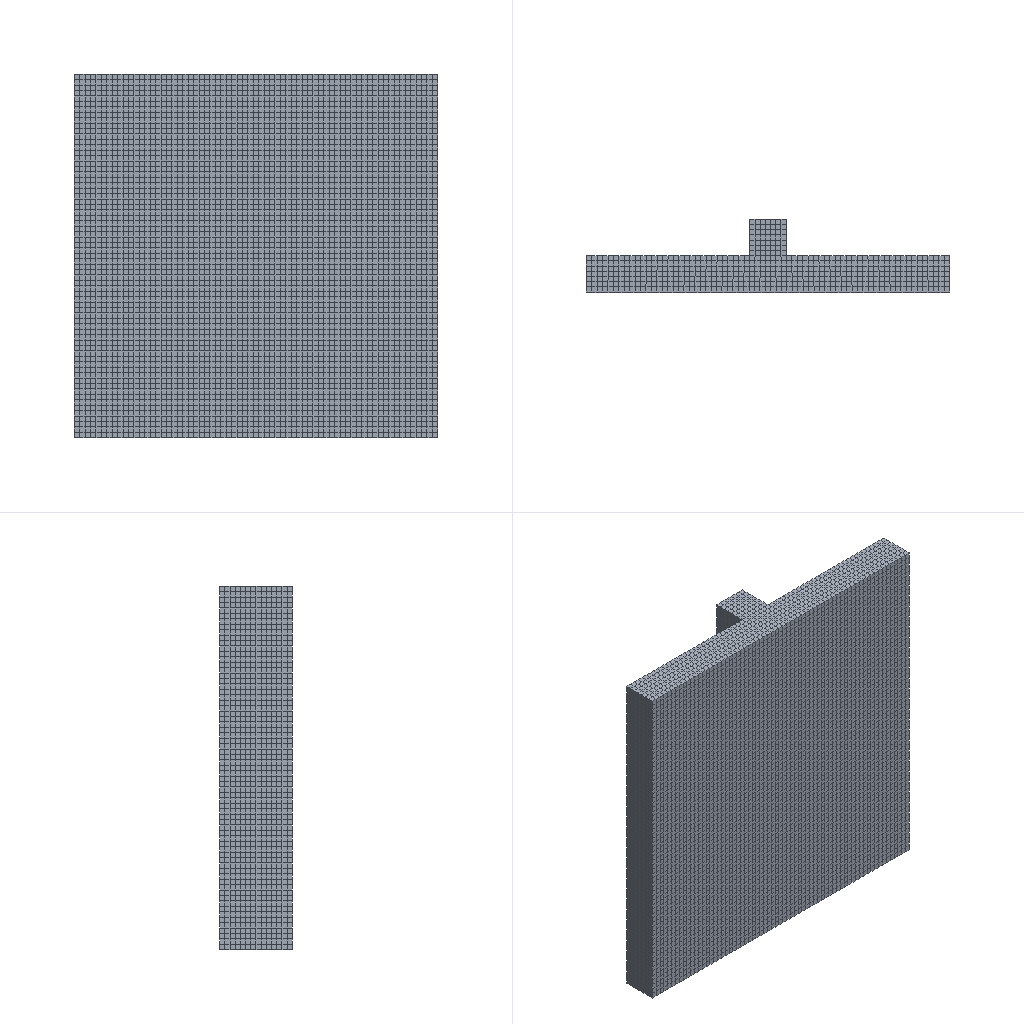Simulation study | abaqus
Set-up summary, first 153 of 190 lines:
category,name,step,type,value,unit,region
solver,abaqus,,Abaqus/CAE 2024
units,mm-N-s-tonne (MPa),,inferred,E= density=7.8e-09
analysis,Step-1,,heat transfer,time_period=2.76
analysis,Step-2,,heat transfer,time_period=50
mesh,nodes,,,40800
mesh,elements,,,34706
element_type,DC3D8,,,34706
material,Material-1,,density,7.8e-09
material,Material-1,,conductivity,17.5
material,Material-1,,specific_heat,5.13e+08
material,Material-1,,behaviors,conductivity; specific heat
section,Material-1,,solid section,,,Set-1
load,Predefined,initial,initial condition temperature
load,Load-1,Step-1,dflux,3.23768e-290,,Part-1-1.316
load,Load-1,Step-1,dflux,2.36258e-281,,Part-1-1.316
load,Load-1,Step-1,dflux,4.91222e-276,,Part-1-1.316
load,Load-1,Step-1,dflux,2.9101e-274,,Part-1-1.316
load,Load-1,Step-1,dflux,4.91222e-276,,Part-1-1.316
load,Load-1,Step-1,dflux,2.36258e-281,,Part-1-1.316
load,Load-1,Step-1,dflux,3.23768e-290,,Part-1-1.316
load,Load-1,Step-1,dflux,1.0318e-245,,Part-1-1.316
load,Load-1,Step-1,dflux,7.52918e-237,,Part-1-1.316
load,Load-1,Step-1,dflux,1.56545e-231,,Part-1-1.316
load,Load-1,Step-1,dflux,9.27406e-230,,Part-1-1.316
load,Load-1,Step-1,dflux,1.56545e-231,,Part-1-1.316
load,Load-1,Step-1,dflux,7.52918e-237,,Part-1-1.316
load,Load-1,Step-1,dflux,1.0318e-245,,Part-1-1.316
load,Load-1,Step-1,dflux,4.43605e-205,,Part-1-1.316
load,Load-1,Step-1,dflux,3.23705e-196,,Part-1-1.316
load,Load-1,Step-1,dflux,6.7304e-191,,Part-1-1.316
load,Load-1,Step-1,dflux,3.98723e-189,,Part-1-1.316
load,Load-1,Step-1,dflux,6.7304e-191,,Part-1-1.316
load,Load-1,Step-1,dflux,3.23705e-196,,Part-1-1.316
load,Load-1,Step-1,dflux,4.43605e-205,,Part-1-1.316
load,Load-1,Step-1,dflux,2.57396e-168,,Part-1-1.316
load,Load-1,Step-1,dflux,1.87825e-159,,Part-1-1.316
load,Load-1,Step-1,dflux,3.90522e-154,,Part-1-1.316
load,Load-1,Step-1,dflux,2.31353e-152,,Part-1-1.316
load,Load-1,Step-1,dflux,3.90522e-154,,Part-1-1.316
load,Load-1,Step-1,dflux,1.87825e-159,,Part-1-1.316
load,Load-1,Step-1,dflux,2.57396e-168,,Part-1-1.316
load,Load-1,Step-1,dflux,2.01555e-135,,Part-1-1.316
load,Load-1,Step-1,dflux,1.47078e-126,,Part-1-1.316
load,Load-1,Step-1,dflux,3.05801e-121,,Part-1-1.316
load,Load-1,Step-1,dflux,1.81163e-119,,Part-1-1.316
load,Load-1,Step-1,dflux,3.05801e-121,,Part-1-1.316
load,Load-1,Step-1,dflux,1.47078e-126,,Part-1-1.316
load,Load-1,Step-1,dflux,2.01555e-135,,Part-1-1.316
load,Load-1,Step-1,dflux,2.12957e-106,,Part-1-1.316
load,Load-1,Step-1,dflux,1.55398e-97,,Part-1-1.316
load,Load-1,Step-1,dflux,3.231e-92,,Part-1-1.316
load,Load-1,Step-1,dflux,1.91411e-90,,Part-1-1.316
load,Load-1,Step-1,dflux,3.231e-92,,Part-1-1.316
load,Load-1,Step-1,dflux,1.55398e-97,,Part-1-1.316
load,Load-1,Step-1,dflux,2.12957e-106,,Part-1-1.316
load,Load-1,Step-1,dflux,3.03647e-81,,Part-1-1.316
load,Load-1,Step-1,dflux,2.21575e-72,,Part-1-1.316
load,Load-1,Step-1,dflux,4.60694e-67,,Part-1-1.316
load,Load-1,Step-1,dflux,2.72925e-65,,Part-1-1.316
load,Load-1,Step-1,dflux,4.60694e-67,,Part-1-1.316
load,Load-1,Step-1,dflux,2.21575e-72,,Part-1-1.316
load,Load-1,Step-1,dflux,3.03647e-81,,Part-1-1.316
load,Load-1,Step-1,dflux,5.84197e-60,,Part-1-1.316
load,Load-1,Step-1,dflux,4.26297e-51,,Part-1-1.316
load,Load-1,Step-1,dflux,8.86347e-46,,Part-1-1.316
load,Load-1,Step-1,dflux,5.2509e-44,,Part-1-1.316
load,Load-1,Step-1,dflux,8.86347e-46,,Part-1-1.316
load,Load-1,Step-1,dflux,4.26297e-51,,Part-1-1.316
load,Load-1,Step-1,dflux,5.84197e-60,,Part-1-1.316
load,Load-1,Step-1,dflux,1.5167e-42,,Part-1-1.316
load,Load-1,Step-1,dflux,1.10676e-33,,Part-1-1.316
load,Load-1,Step-1,dflux,2.30114e-28,,Part-1-1.316
load,Load-1,Step-1,dflux,1.36324e-26,,Part-1-1.316
load,Load-1,Step-1,dflux,2.30114e-28,,Part-1-1.316
load,Load-1,Step-1,dflux,1.10676e-33,,Part-1-1.316
load,Load-1,Step-1,dflux,1.5167e-42,,Part-1-1.316
load,Load-1,Step-1,dflux,5.31377e-29,,Part-1-1.316
load,Load-1,Step-1,dflux,3.87753e-20,,Part-1-1.316
load,Load-1,Step-1,dflux,8.06207e-15,,Part-1-1.316
load,Load-1,Step-1,dflux,4.77614e-13,,Part-1-1.316
load,Load-1,Step-1,dflux,8.06207e-15,,Part-1-1.316
load,Load-1,Step-1,dflux,3.87753e-20,,Part-1-1.316
load,Load-1,Step-1,dflux,5.31377e-29,,Part-1-1.316
load,Load-1,Step-1,dflux,2.51209e-19,,Part-1-1.316
load,Load-1,Step-1,dflux,1.83311e-10,,Part-1-1.316
load,Load-1,Step-1,dflux,3.81135e-05,,Part-1-1.316
load,Load-1,Step-1,dflux,0.002258,,Part-1-1.316
load,Load-1,Step-1,dflux,3.81135e-05,,Part-1-1.316
load,Load-1,Step-1,dflux,1.83311e-10,,Part-1-1.316
load,Load-1,Step-1,dflux,2.51209e-19,,Part-1-1.316
load,Load-1,Step-1,dflux,1.60257e-13,,Part-1-1.316
load,Load-1,Step-1,dflux,0.0001169,,Part-1-1.316
load,Load-1,Step-1,dflux,24.314,,Part-1-1.317
load,Load-1,Step-1,dflux,1440.43,,Part-1-1.317
load,Load-1,Step-1,dflux,24.314,,Part-1-1.317
load,Load-1,Step-1,dflux,0.0001169,,Part-1-1.317
load,Load-1,Step-1,dflux,1.60257e-13,,Part-1-1.317
load,Load-1,Step-1,dflux,1.37958e-11,,Part-1-1.317
load,Load-1,Step-1,dflux,0.01007,,Part-1-1.317
load,Load-1,Step-1,dflux,2093.11,,Part-1-1.317
load,Load-1,Step-1,dflux,124000,,Part-1-1.317
load,Load-1,Step-1,dflux,2093.11,,Part-1-1.317
load,Load-1,Step-1,dflux,0.01007,,Part-1-1.317
load,Load-1,Step-1,dflux,1.37958e-11,,Part-1-1.317
load,Load-1,Step-1,dflux,1.60257e-13,,Part-1-1.317
load,Load-1,Step-1,dflux,0.0001169,,Part-1-1.317
load,Load-1,Step-1,dflux,24.314,,Part-1-1.317
load,Load-1,Step-1,dflux,1440.43,,Part-1-1.317
load,Load-1,Step-1,dflux,24.314,,Part-1-1.317
load,Load-1,Step-1,dflux,0.0001169,,Part-1-1.317
load,Load-1,Step-1,dflux,1.60257e-13,,Part-1-1.317
load,Load-1,Step-1,dflux,2.51209e-19,,Part-1-1.317
load,Load-1,Step-1,dflux,1.83311e-10,,Part-1-1.317
load,Load-1,Step-1,dflux,3.81135e-05,,Part-1-1.317
load,Load-1,Step-1,dflux,0.002258,,Part-1-1.317
load,Load-1,Step-1,dflux,3.81135e-05,,Part-1-1.317
load,Load-1,Step-1,dflux,1.83311e-10,,Part-1-1.317
load,Load-1,Step-1,dflux,2.51209e-19,,Part-1-1.317
load,Load-1,Step-1,dflux,5.31377e-29,,Part-1-1.317
load,Load-1,Step-1,dflux,3.87753e-20,,Part-1-1.317
load,Load-1,Step-1,dflux,8.06207e-15,,Part-1-1.317
load,Load-1,Step-1,dflux,4.77614e-13,,Part-1-1.317
load,Load-1,Step-1,dflux,8.06207e-15,,Part-1-1.317
load,Load-1,Step-1,dflux,3.87753e-20,,Part-1-1.317
load,Load-1,Step-1,dflux,5.31377e-29,,Part-1-1.317
load,Load-1,Step-1,dflux,1.5167e-42,,Part-1-1.317
load,Load-1,Step-1,dflux,1.10676e-33,,Part-1-1.317
load,Load-1,Step-1,dflux,2.30114e-28,,Part-1-1.317
load,Load-1,Step-1,dflux,1.36324e-26,,Part-1-1.317
load,Load-1,Step-1,dflux,2.30114e-28,,Part-1-1.317
load,Load-1,Step-1,dflux,1.10676e-33,,Part-1-1.317
load,Load-1,Step-1,dflux,1.5167e-42,,Part-1-1.317
load,Load-1,Step-1,dflux,5.84197e-60,,Part-1-1.317
load,Load-1,Step-1,dflux,4.26297e-51,,Part-1-1.317
load,Load-1,Step-1,dflux,8.86347e-46,,Part-1-1.317
load,Load-1,Step-1,dflux,5.2509e-44,,Part-1-1.317
load,Load-1,Step-1,dflux,8.86347e-46,,Part-1-1.317
load,Load-1,Step-1,dflux,4.26297e-51,,Part-1-1.317
load,Load-1,Step-1,dflux,5.84197e-60,,Part-1-1.317
load,Load-1,Step-1,dflux,3.03647e-81,,Part-1-1.317
load,Load-1,Step-1,dflux,2.21575e-72,,Part-1-1.317
load,Load-1,Step-1,dflux,4.60694e-67,,Part-1-1.317
load,Load-1,Step-1,dflux,2.72925e-65,,Part-1-1.317
load,Load-1,Step-1,dflux,4.60694e-67,,Part-1-1.317
load,Load-1,Step-1,dflux,2.21575e-72,,Part-1-1.317
load,Load-1,Step-1,dflux,3.03647e-81,,Part-1-1.317
load,Load-1,Step-1,dflux,2.12957e-106,,Part-1-1.317
load,Load-1,Step-1,dflux,1.55398e-97,,Part-1-1.317
load,Load-1,Step-1,dflux,3.231e-92,,Part-1-1.317
load,Load-1,Step-1,dflux,1.91411e-90,,Part-1-1.317
load,Load-1,Step-1,dflux,3.231e-92,,Part-1-1.317
load,Load-1,Step-1,dflux,1.55398e-97,,Part-1-1.317
Abaqus input file, long lists of numbers shortened:
*Heading
** Job name: deck Model name: Model-1
** Generated by: Abaqus/CAE 2024
*Preprint, echo=NO, model=NO, history=NO, contact=NO
**
** PARTS
**
*Part, name=Part-1
*Node
      1,          50.,         -10.,         100.
      2,         -50.,         -10.,         100.
** (40798 more lines like these left out)
*Element, type=DC3D8
    1,   684, 10237, 12289,  9445,     1,    17,   865,   280
    2, 10237, 10238, 12290, 12289,    17,    18,   866,   865
** (34704 more lines like these left out)
*Nset, nset=Set-1, generate
     1,  40800,      1
*Elset, elset=Set-1, generate
     1,  34706,      1
** Section: Section-1
*Solid Section, elset=Set-1, material=Material-1
,
*End Part
**
**
** ASSEMBLY
**
*Assembly, name=Assembly
**
*Instance, name=Part-1-1, part=Part-1
*End Instance
**
*Nset, nset=Set-1, instance=Part-1-1, generate
     1,  40800,      1
*Elset, elset=Set-1, instance=Part-1-1, generate
     1,  34706,      1
*Elset, elset=_Surf-1_S6, internal, instance=Part-1-1
     1,    68,   135,   202,   269,   336,   403,   470,   537,   604,   671,   738,   805,   872,   939,  1006
  1073,  1140,  1207,  1274,  1341,  1408,  1475,  1542,  1609,  1676,  1743,  1810,  1877,  1944,  2011,  2078
** (57 more lines like these left out)
*Elset, elset=_Surf-1_S2, internal, instance=Part-1-1
     1,     2,     3,     4,     5,     6,     7,     8,     9,    10,    11,    12,    13,    14,    15,    16
    17,    18,    19,    20,    21,    22,    23,    24,    25,    26,    27,    28,    29,    30,    31,    32
** (308 more lines like these left out)
*Elset, elset=_Surf-1_S4, internal, instance=Part-1-1
    67,   134,   201,   268,   335,   402,   469,   536,   603,   670,   737,   804,   871,   938,  1005,  1072
  1139,  1206,  1273,  1340,  1407,  1474,  1541,  1608,  1675,  1742,  1809,  1876,  1943,  2010,  2077,  2144
** (57 more lines like these left out)
*Elset, elset=_Surf-1_S1, internal, instance=Part-1-1
 26935, 26936, 26937, 26938, 26939, 26940, 26941, 26942, 26943, 26944, 26945, 26946, 26947, 26948, 26949, 26950
 26951, 26952, 26953, 26954, 26955, 26956, 26957, 26958, 26959, 26960, 26961, 26962, 26963, 26964, 26972, 26973
** (250 more lines like these left out)
*Elset, elset=_Surf-1_S3, internal, instance=Part-1-1
     1,     2,     3,     4,     5,     6,     7,     8,     9,    10,    11,    12,    13,    14,    15,    16
    17,    18,    19,    20,    21,    22,    23,    24,    25,    26,    27,    28,    29,    30,    31,    32
** (31 more lines like these left out)
*Elset, elset=_Surf-1_S5, internal, instance=Part-1-1
  4423,  4424,  4425,  4426,  4427,  4428,  4429,  4430,  4431,  4432,  4433,  4434,  4435,  4436,  4437,  4438
  4439,  4440,  4441,  4442,  4443,  4444,  4445,  4446,  4447,  4448,  4449,  4450,  4451,  4452,  4453,  4454
** (31 more lines like these left out)
*Surface, type=ELEMENT, name=Surf-1
_Surf-1_S6, S6
_Surf-1_S2, S2
_Surf-1_S4, S4
_Surf-1_S1, S1
_Surf-1_S3, S3
_Surf-1_S5, S5
*Elset, elset=_Surf-2_S2, internal, instance=Part-1-1, generate
 31424,  31892,      1
*Surface, type=ELEMENT, name=Surf-2
_Surf-2_S2, S2
*Elset, elset=_Surf-3_S5, internal, instance=Part-1-1
  4423,  4424,  4425,  4426,  4427,  4428,  4429,  4430,  4431,  4432,  4433,  4434,  4435,  4436,  4437,  4438
  4439,  4440,  4441,  4442,  4443,  4444,  4445,  4446,  4447,  4448,  4449,  4450,  4451,  4452,  4453,  4454
** (31 more lines like these left out)
*Elset, elset=_Surf-3_S3, internal, instance=Part-1-1
     1,     2,     3,     4,     5,     6,     7,     8,     9,    10,    11,    12,    13,    14,    15,    16
    17,    18,    19,    20,    21,    22,    23,    24,    25,    26,    27,    28,    29,    30,    31,    32
** (31 more lines like these left out)
*Elset, elset=_Surf-3_S6, internal, instance=Part-1-1
     1,    68,   135,   202,   269,   336,   403,   470,   537,   604,   671,   738,   805,   872,   939,  1006
  1073,  1140,  1207,  1274,  1341,  1408,  1475,  1542,  1609,  1676,  1743,  1810,  1877,  1944,  2011,  2078
** (57 more lines like these left out)
*Elset, elset=_Surf-3_S2, internal, instance=Part-1-1
     1,     2,     3,     4,     5,     6,     7,     8,     9,    10,    11,    12,    13,    14,    15,    16
    17,    18,    19,    20,    21,    22,    23,    24,    25,    26,    27,    28,    29,    30,    31,    32
** (308 more lines like these left out)
*Elset, elset=_Surf-3_S4, internal, instance=Part-1-1
    67,   134,   201,   268,   335,   402,   469,   536,   603,   670,   737,   804,   871,   938,  1005,  1072
  1139,  1206,  1273,  1340,  1407,  1474,  1541,  1608,  1675,  1742,  1809,  1876,  1943,  2010,  2077,  2144
** (57 more lines like these left out)
*Elset, elset=_Surf-3_S1, internal, instance=Part-1-1
 26935, 26936, 26937, 26938, 26939, 26940, 26941, 26942, 26943, 26944, 26945, 26946, 26947, 26948, 26949, 26950
 26951, 26952, 26953, 26954, 26955, 26956, 26957, 26958, 26959, 26960, 26961, 26962, 26963, 26964, 26972, 26973
** (250 more lines like these left out)
*Surface, type=ELEMENT, name=Surf-3
_Surf-3_S5, S5
_Surf-3_S3, S3
_Surf-3_S6, S6
_Surf-3_S2, S2
_Surf-3_S4, S4
_Surf-3_S1, S1
*End Assembly
**
** MATERIALS
**
*Material, name=Material-1
*Conductivity
 17.5,
*Density
 7.8e-09,
*Specific Heat
 5.13e+08,
**
** PREDEFINED FIELDS
**
** Name: Predefined Field-1   Type: Temperature
*Initial Conditions, type=TEMPERATURE
Set-1, 20.
** ----------------------------------------------------------------
**
** STEP: Step-1
**
*Step, name=Step-1, nlgeom=NO, inc=1000
*Heat Transfer, end=PERIOD, deltmx=800.
0.01, 2.76, 2.76e-05, 2.76,
**
** LOADS
**
** Name: Load-1   Type: Surface heat flux Using Field: AnalyticalField-1
*Dflux
Part-1-1.316, S2, 3.23768e-290
Part-1-1.316, S2, 2.36258e-281
Part-1-1.316, S2, 4.91222e-276
Part-1-1.316, S2, 2.9101e-274
Part-1-1.316, S2, 4.91222e-276
Part-1-1.316, S2, 2.36258e-281
Part-1-1.316, S2, 3.23768e-290
Part-1-1.316, S2, 1.0318e-245
Part-1-1.316, S2, 7.52918e-237
Part-1-1.316, S2, 1.56545e-231
Part-1-1.316, S2, 9.27406e-230
Part-1-1.316, S2, 1.56545e-231
Part-1-1.316, S2, 7.52918e-237
Part-1-1.316, S2, 1.0318e-245
Part-1-1.316, S2, 4.43605e-205
Part-1-1.316, S2, 3.23705e-196
Part-1-1.316, S2, 6.7304e-191
Part-1-1.316, S2, 3.98723e-189
Part-1-1.316, S2, 6.7304e-191
Part-1-1.316, S2, 3.23705e-196
Part-1-1.316, S2, 4.43605e-205
Part-1-1.316, S2, 2.57396e-168
Part-1-1.316, S2, 1.87825e-159
Part-1-1.316, S2, 3.90522e-154
Part-1-1.316, S2, 2.31353e-152
Part-1-1.316, S2, 3.90522e-154
Part-1-1.316, S2, 1.87825e-159
Part-1-1.316, S2, 2.57396e-168
Part-1-1.316, S2, 2.01555e-135
Part-1-1.316, S2, 1.47078e-126
Part-1-1.316, S2, 3.05801e-121
Part-1-1.316, S2, 1.81163e-119
Part-1-1.316, S2, 3.05801e-121
Part-1-1.316, S2, 1.47078e-126
Part-1-1.316, S2, 2.01555e-135
Part-1-1.316, S2, 2.12957e-106
Part-1-1.316, S2, 1.55398e-97
Part-1-1.316, S2, 3.231e-92
Part-1-1.316, S2, 1.91411e-90
Part-1-1.316, S2, 3.231e-92
** (135 more lines like these left out)
**
** INTERACTIONS
**
** Interaction: Int-1
*Sfilm
Surf-3, F, 20., 0.2
**
** OUTPUT REQUESTS
**
*Restart, write, frequency=0
**
** FIELD OUTPUT: F-Output-1
**
*Output, field, variable=PRESELECT
*Output, history, frequency=0
*End Step
** ----------------------------------------------------------------
**
** STEP: Step-2
**
*Step, name=Step-2, nlgeom=NO, inc=10000
*Heat Transfer, end=PERIOD, deltmx=800.
0.05, 50., 0.0005, 50.,
**
** LOADS
**
** Name: Load-1   Type: Surface heat flux Using Field: AnalyticalField-1
*Dflux, op=NEW
**
** OUTPUT REQUESTS
**
*Restart, write, frequency=0
**
** FIELD OUTPUT: F-Output-1
**
*Output, field, variable=PRESELECT
*Output, history, frequency=0
*End Step
Results summary:
result,odb.job_status,,,JOB_STATUS_COMPLETED_SUCCESSFULLY,"consistent, unstated (Abaqus has no unit system)"
result,steps[0].procedure,Step-1,,"*HEAT TRANSFER, DELTAMX","consistent, unstated (Abaqus has no unit system)"
result,steps[0].time_period,Step-1,,2.76,"consistent, unstated (Abaqus has no unit system)"
result,steps[0].n_frames,Step-1,,15,"consistent, unstated (Abaqus has no unit system)"
result,steps[0].last_frame.id,Step-1,,14,"consistent, unstated (Abaqus has no unit system)"
result,steps[0].last_frame.value,Step-1,,2.76,"consistent, unstated (Abaqus has no unit system)"
result,steps[0].last_frame.description,Step-1,,Increment     14: Step Time =    2.760,"consistent, unstated (Abaqus has no unit system)"
result,steps[0].completed,Step-1,,True,"consistent, unstated (Abaqus has no unit system)"
result,steps[1].procedure,Step-2,,"*HEAT TRANSFER, DELTAMX","consistent, unstated (Abaqus has no unit system)"
result,steps[1].time_period,Step-2,,50,"consistent, unstated (Abaqus has no unit system)"
result,steps[1].n_frames,Step-2,,17,"consistent, unstated (Abaqus has no unit system)"
result,steps[1].last_frame.id,Step-2,,16,"consistent, unstated (Abaqus has no unit system)"
result,steps[1].last_frame.value,Step-2,,50,"consistent, unstated (Abaqus has no unit system)"
result,steps[1].last_frame.description,Step-2,,Increment     16: Step Time =    50.00,"consistent, unstated (Abaqus has no unit system)"
result,steps[1].completed,Step-2,,True,"consistent, unstated (Abaqus has no unit system)"